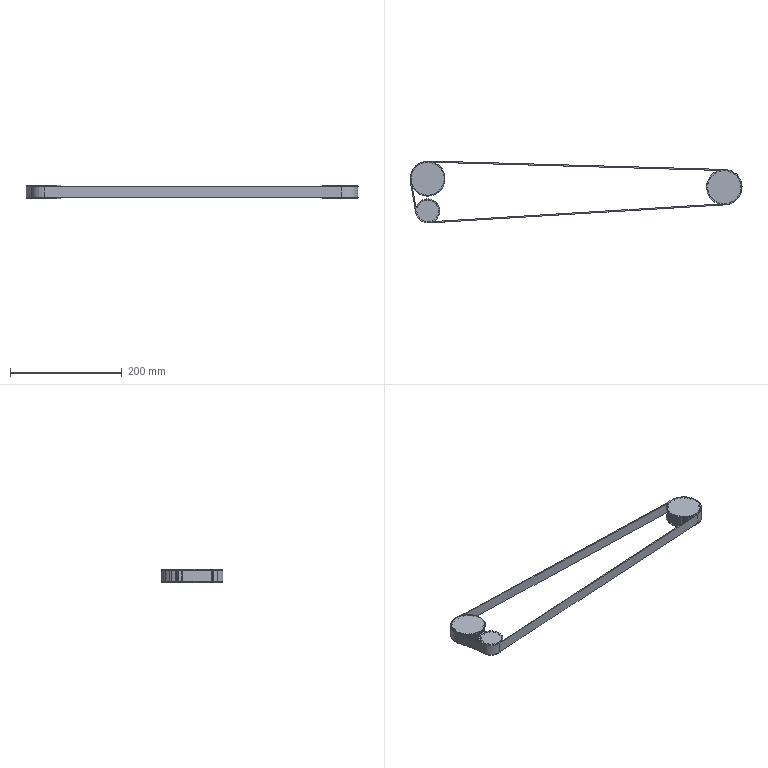Part | SolidWorks | 4 solids | 629 faces | box 593.838 x 110.876 x 23.437 mm | volume 192457 mm3 | cylinder 367 | plane 214 | cone 36 | torus 12 | commonest cylinder face diameters 3.2 x320 59.266 x32 39.054 x12 63.33 x2 43.118 x1